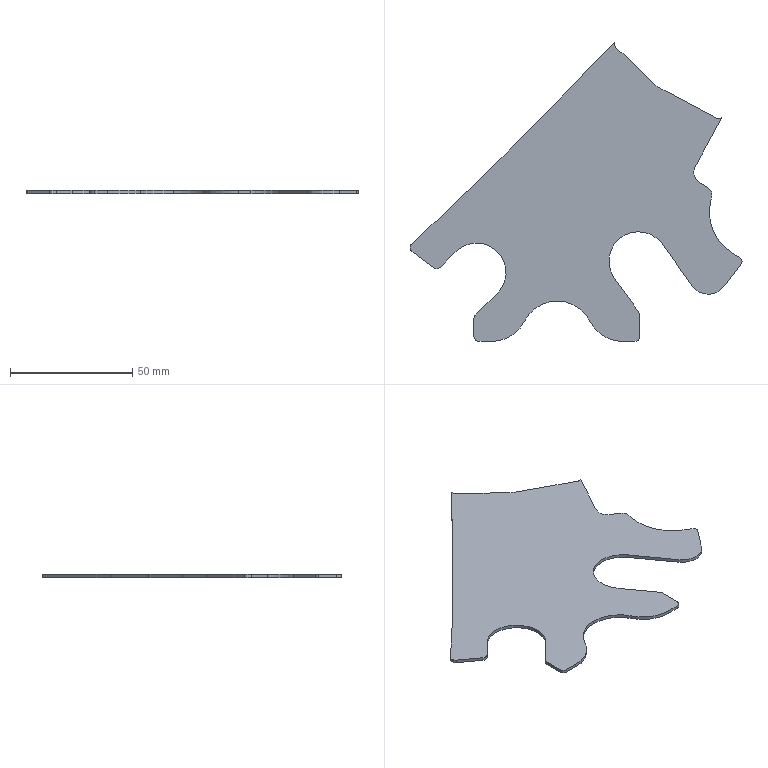Part | STEP file | gslz 2016.10.28-13_id214_x_t | 1 solid | 45 faces | box 135.694 x 122.174 x 1.25 mm | volume 10095 mm3 | plane 24 | cylinder 21 | commonest cylinder face diameters 4 x9 30 x4 16 x2 24 x2 40 x2 6 x1